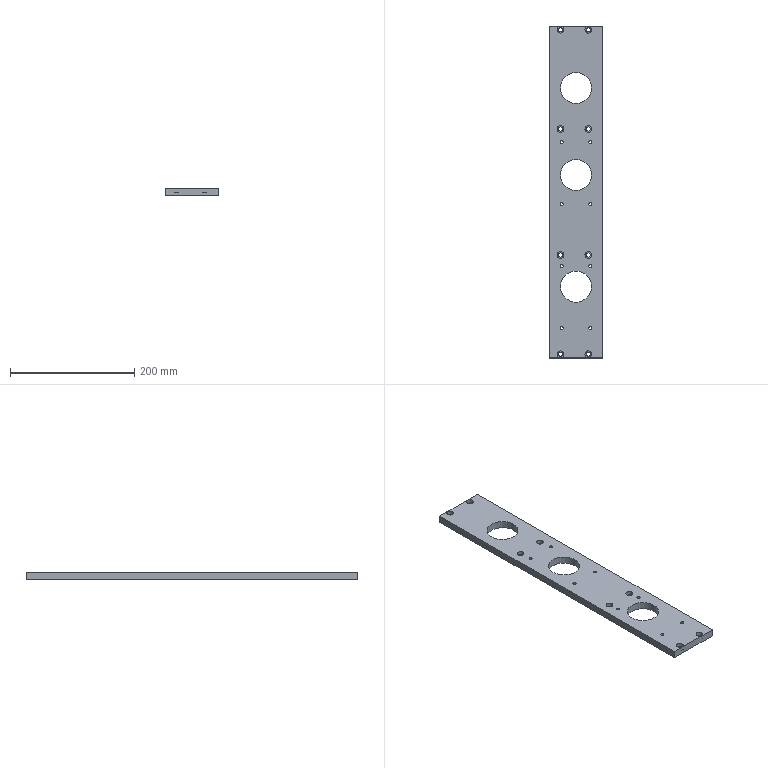Part | NX | 1 solid | 51 faces | box 86 x 535 x 12 mm | volume 472152 mm3 | cylinder 32 | plane 14 | cone 5 | commonest cylinder face diameters 5 x8 6.6 x8 11 x8 4.2 x5 50 x3
STEP:
#1=CARTESIAN_POINT('',(43.,-257.5,-2.1));
#2=VERTEX_POINT('',#1);
#3=CARTESIAN_POINT('',(43.,-257.5,0.));
#4=DIRECTION('',(1.,0.,0.));
#5=DIRECTION('',(0.,0.,-1.));
#6=AXIS2_PLACEMENT_3D('',#3,#4,#5);
#7=CIRCLE('',#6,2.1);
#8=EDGE_CURVE('',#2,#2,#7,.T.);
#9=ORIENTED_EDGE('',*,*,#8,.F.);
#10=EDGE_LOOP('',(#9));
#11=FACE_BOUND('',#10,.T.);
#12=CARTESIAN_POINT('',(43.,-117.5,-2.1));
#13=VERTEX_POINT('',#12);
#14=CARTESIAN_POINT('',(43.,-117.5,0.));
#15=DIRECTION('',(1.,0.,0.));
#16=DIRECTION('',(0.,0.,-1.));
#17=AXIS2_PLACEMENT_3D('',#14,#15,#16);
#18=CIRCLE('',#17,2.1);
#19=EDGE_CURVE('',#13,#13,#18,.T.);
#20=ORIENTED_EDGE('',*,*,#19,.F.);
#21=EDGE_LOOP('',(#20));
#22=FACE_BOUND('',#21,.T.);
#23=CARTESIAN_POINT('',(43.,117.5,-2.1));
#24=VERTEX_POINT('',#23);
#25=CARTESIAN_POINT('',(43.,117.5,0.));
#26=DIRECTION('',(1.,0.,0.));
#27=DIRECTION('',(0.,0.,-1.));
#28=AXIS2_PLACEMENT_3D('',#25,#26,#27);
#29=CIRCLE('',#28,2.1);
#30=EDGE_CURVE('',#24,#24,#29,.T.);
#31=ORIENTED_EDGE('',*,*,#30,.F.);
#32=EDGE_LOOP('',(#31));
#33=FACE_BOUND('',#32,.T.);
#34=CARTESIAN_POINT('',(43.,257.5,-2.1));
#35=VERTEX_POINT('',#34);
#36=CARTESIAN_POINT('',(43.,257.5,0.));
#37=DIRECTION('',(1.,0.,0.));
#38=DIRECTION('',(0.,0.,-1.));
#39=AXIS2_PLACEMENT_3D('',#36,#37,#38);
#40=CIRCLE('',#39,2.1);
#41=EDGE_CURVE('',#35,#35,#40,.T.);
#42=ORIENTED_EDGE('',*,*,#41,.F.);
#43=EDGE_LOOP('',(#42));
#44=FACE_BOUND('',#43,.T.);
#45=CARTESIAN_POINT('',(43.,0.,-2.1));
#46=VERTEX_POINT('',#45);
#47=CARTESIAN_POINT('',(43.,0.,0.));
#48=DIRECTION('',(1.,0.,0.));
#49=DIRECTION('',(0.,0.,-1.));
#50=AXIS2_PLACEMENT_3D('',#47,#48,#49);
#51=CIRCLE('',#50,2.1);
#52=EDGE_CURVE('',#46,#46,#51,.T.);
#53=ORIENTED_EDGE('',*,*,#52,.F.);
#54=EDGE_LOOP('',(#53));
#55=FACE_BOUND('',#54,.T.);
#56=CARTESIAN_POINT('',(43.,-267.5,-6.));
#57=VERTEX_POINT('',#56);
#58=CARTESIAN_POINT('',(43.,267.5,-6.));
#59=VERTEX_POINT('',#58);
#60=CARTESIAN_POINT('',(43.,267.5,-6.));
#61=DIRECTION('',(0.,1.,0.));
#62=VECTOR('',#61,1000.);
#63=LINE('',#60,#62);
#64=EDGE_CURVE('',#57,#59,#63,.T.);
#65=ORIENTED_EDGE('',*,*,#64,.T.);
#66=CARTESIAN_POINT('',(43.,267.5,6.));
#67=VERTEX_POINT('',#66);
#68=CARTESIAN_POINT('',(43.,267.5,6.));
#69=DIRECTION('',(0.,0.,-1.));
#70=VECTOR('',#69,1000.);
#71=LINE('',#68,#70);
#72=EDGE_CURVE('',#67,#59,#71,.T.);
#73=ORIENTED_EDGE('',*,*,#72,.F.);
#74=CARTESIAN_POINT('',(43.,-267.5,6.));
#75=VERTEX_POINT('',#74);
#76=CARTESIAN_POINT('',(43.,267.5,6.));
#77=DIRECTION('',(0.,1.,0.));
#78=VECTOR('',#77,1000.);
#79=LINE('',#76,#78);
#80=EDGE_CURVE('',#75,#67,#79,.T.);
#81=ORIENTED_EDGE('',*,*,#80,.F.);
#82=CARTESIAN_POINT('',(43.,-267.5,6.));
#83=DIRECTION('',(0.,0.,-1.));
#84=VECTOR('',#83,1000.);
#85=LINE('',#82,#84);
#86=EDGE_CURVE('',#75,#57,#85,.T.);
#87=ORIENTED_EDGE('',*,*,#86,.T.);
#88=EDGE_LOOP('',(#65,#73,#81,#87));
#89=FACE_BOUND('',#88,.T.);
#90=CARTESIAN_POINT('',(43.,267.5,6.));
#91=DIRECTION('',(-1.,0.,0.));
#92=DIRECTION('',(0.,-1.,0.));
#93=AXIS2_PLACEMENT_3D('',#90,#91,#92);
#94=PLANE('',#93);
#95=ADVANCED_FACE('',(#11,#22,#33,#44,#55,#89),#94,.F.);
#96=CARTESIAN_POINT('',(-43.,267.5,-6.));
#97=VERTEX_POINT('',#96);
#98=CARTESIAN_POINT('',(-43.,267.5,-6.));
#99=DIRECTION('',(-1.,0.,0.));
#100=VECTOR('',#99,1000.);
#101=LINE('',#98,#100);
#102=EDGE_CURVE('',#59,#97,#101,.T.);
#103=ORIENTED_EDGE('',*,*,#102,.T.);
#104=CARTESIAN_POINT('',(-43.,267.5,6.));
#105=VERTEX_POINT('',#104);
#106=CARTESIAN_POINT('',(-43.,267.5,6.));
#107=DIRECTION('',(0.,0.,-1.));
#108=VECTOR('',#107,1000.);
#109=LINE('',#106,#108);
#110=EDGE_CURVE('',#105,#97,#109,.T.);
#111=ORIENTED_EDGE('',*,*,#110,.F.);
#112=CARTESIAN_POINT('',(-43.,267.5,6.));
#113=DIRECTION('',(-1.,0.,0.));
#114=VECTOR('',#113,1000.);
#115=LINE('',#112,#114);
#116=EDGE_CURVE('',#67,#105,#115,.T.);
#117=ORIENTED_EDGE('',*,*,#116,.F.);
#118=ORIENTED_EDGE('',*,*,#72,.T.);
#119=EDGE_LOOP('',(#103,#111,#117,#118));
#120=FACE_BOUND('',#119,.T.);
#121=CARTESIAN_POINT('',(-43.,267.5,6.));
#122=DIRECTION('',(0.,-1.,0.));
#123=DIRECTION('',(0.,0.,-1.));
#124=AXIS2_PLACEMENT_3D('',#121,#122,#123);
#125=PLANE('',#124);
#126=ADVANCED_FACE('',(#120),#125,.F.);
#127=CARTESIAN_POINT('',(-43.,-267.5,-6.));
#128=VERTEX_POINT('',#127);
#129=CARTESIAN_POINT('',(-43.,267.5,-6.));
#130=DIRECTION('',(0.,-1.,0.));
#131=VECTOR('',#130,1000.);
#132=LINE('',#129,#131);
#133=EDGE_CURVE('',#97,#128,#132,.T.);
#134=ORIENTED_EDGE('',*,*,#133,.T.);
#135=CARTESIAN_POINT('',(-43.,-267.5,6.));
#136=VERTEX_POINT('',#135);
#137=CARTESIAN_POINT('',(-43.,-267.5,6.));
#138=DIRECTION('',(0.,0.,-1.));
#139=VECTOR('',#138,1000.);
#140=LINE('',#137,#139);
#141=EDGE_CURVE('',#136,#128,#140,.T.);
#142=ORIENTED_EDGE('',*,*,#141,.F.);
#143=CARTESIAN_POINT('',(-43.,267.5,6.));
#144=DIRECTION('',(0.,-1.,0.));
#145=VECTOR('',#144,1000.);
#146=LINE('',#143,#145);
#147=EDGE_CURVE('',#105,#136,#146,.T.);
#148=ORIENTED_EDGE('',*,*,#147,.F.);
#149=ORIENTED_EDGE('',*,*,#110,.T.);
#150=EDGE_LOOP('',(#134,#142,#148,#149));
#151=FACE_BOUND('',#150,.T.);
#152=CARTESIAN_POINT('',(-43.,267.5,6.));
#153=DIRECTION('',(1.,0.,0.));
#154=DIRECTION('',(0.,1.,0.));
#155=AXIS2_PLACEMENT_3D('',#152,#153,#154);
#156=PLANE('',#155);
#157=ADVANCED_FACE('',(#151),#156,.F.);
#158=CARTESIAN_POINT('',(-43.,-267.5,-6.));
#159=DIRECTION('',(1.,0.,0.));
#160=VECTOR('',#159,1000.);
#161=LINE('',#158,#160);
#162=EDGE_CURVE('',#128,#57,#161,.T.);
#163=ORIENTED_EDGE('',*,*,#162,.T.);
#164=ORIENTED_EDGE('',*,*,#86,.F.);
#165=CARTESIAN_POINT('',(-43.,-267.5,6.));
#166=DIRECTION('',(1.,0.,0.));
#167=VECTOR('',#166,1000.);
#168=LINE('',#165,#167);
#169=EDGE_CURVE('',#136,#75,#168,.T.);
#170=ORIENTED_EDGE('',*,*,#169,.F.);
#171=ORIENTED_EDGE('',*,*,#141,.T.);
#172=EDGE_LOOP('',(#163,#164,#170,#171));
#173=FACE_BOUND('',#172,.T.);
#174=CARTESIAN_POINT('',(-43.,-267.5,6.));
#175=DIRECTION('',(0.,1.,0.));
#176=DIRECTION('',(0.,0.,1.));
#177=AXIS2_PLACEMENT_3D('',#174,#175,#176);
#178=PLANE('',#177);
#179=ADVANCED_FACE('',(#173),#178,.F.);
#180=CARTESIAN_POINT('',(-25.,-152.5,6.));
#181=VERTEX_POINT('',#180);
#182=CARTESIAN_POINT('',(0.,-152.5,6.));
#183=DIRECTION('',(0.,0.,-1.));
#184=DIRECTION('',(-1.,0.,0.));
#185=AXIS2_PLACEMENT_3D('',#182,#183,#184);
#186=CIRCLE('',#185,25.);
#187=EDGE_CURVE('',#181,#181,#186,.T.);
#188=ORIENTED_EDGE('',*,*,#187,.T.);
#189=EDGE_LOOP('',(#188));
#190=FACE_BOUND('',#189,.T.);
#191=CARTESIAN_POINT('',(-25.,27.5,6.));
#192=VERTEX_POINT('',#191);
#193=CARTESIAN_POINT('',(0.,27.5,6.));
#194=DIRECTION('',(0.,0.,-1.));
#195=DIRECTION('',(-1.,0.,0.));
#196=AXIS2_PLACEMENT_3D('',#193,#194,#195);
#197=CIRCLE('',#196,25.);
#198=EDGE_CURVE('',#192,#192,#197,.T.);
#199=ORIENTED_EDGE('',*,*,#198,.T.);
#200=EDGE_LOOP('',(#199));
#201=FACE_BOUND('',#200,.T.);
#202=CARTESIAN_POINT('',(-25.,167.5,6.));
#203=VERTEX_POINT('',#202);
#204=CARTESIAN_POINT('',(0.,167.5,6.));
#205=DIRECTION('',(0.,0.,-1.));
#206=DIRECTION('',(-1.,0.,0.));
#207=AXIS2_PLACEMENT_3D('',#204,#205,#206);
#208=CIRCLE('',#207,25.);
#209=EDGE_CURVE('',#203,#203,#208,.T.);
#210=ORIENTED_EDGE('',*,*,#209,.T.);
#211=EDGE_LOOP('',(#210));
#212=FACE_BOUND('',#211,.T.);
#213=CARTESIAN_POINT('',(-19.5,101.5,6.));
#214=VERTEX_POINT('',#213);
#215=CARTESIAN_POINT('',(-25.,101.5,6.));
#216=DIRECTION('',(0.,0.,1.));
#217=DIRECTION('',(1.,0.,0.));
#218=AXIS2_PLACEMENT_3D('',#215,#216,#217);
#219=CIRCLE('',#218,5.5);
#220=EDGE_CURVE('',#214,#214,#219,.T.);
#221=ORIENTED_EDGE('',*,*,#220,.F.);
#222=EDGE_LOOP('',(#221));
#223=FACE_BOUND('',#222,.T.);
#224=CARTESIAN_POINT('',(25.5,101.5,6.));
#225=VERTEX_POINT('',#224);
#226=CARTESIAN_POINT('',(20.,101.5,6.));
#227=DIRECTION('',(0.,0.,1.));
#228=DIRECTION('',(1.,0.,0.));
#229=AXIS2_PLACEMENT_3D('',#226,#227,#228);
#230=CIRCLE('',#229,5.5);
#231=EDGE_CURVE('',#225,#225,#230,.T.);
#232=ORIENTED_EDGE('',*,*,#231,.F.);
#233=EDGE_LOOP('',(#232));
#234=FACE_BOUND('',#233,.T.);
#235=CARTESIAN_POINT('',(-19.5,-101.5,6.));
#236=VERTEX_POINT('',#235);
#237=CARTESIAN_POINT('',(-25.,-101.5,6.));
#238=DIRECTION('',(0.,0.,1.));
#239=DIRECTION('',(1.,0.,0.));
#240=AXIS2_PLACEMENT_3D('',#237,#238,#239);
#241=CIRCLE('',#240,5.5);
#242=EDGE_CURVE('',#236,#236,#241,.T.);
#243=ORIENTED_EDGE('',*,*,#242,.F.);
#244=EDGE_LOOP('',(#243));
#245=FACE_BOUND('',#244,.T.);
#246=CARTESIAN_POINT('',(25.5,-101.5,6.));
#247=VERTEX_POINT('',#246);
#248=CARTESIAN_POINT('',(20.,-101.5,6.));
#249=DIRECTION('',(0.,0.,1.));
#250=DIRECTION('',(1.,0.,0.));
#251=AXIS2_PLACEMENT_3D('',#248,#249,#250);
#252=CIRCLE('',#251,5.5);
#253=EDGE_CURVE('',#247,#247,#252,.T.);
#254=ORIENTED_EDGE('',*,*,#253,.F.);
#255=EDGE_LOOP('',(#254));
#256=FACE_BOUND('',#255,.T.);
#257=CARTESIAN_POINT('',(-19.5,-261.5,6.));
#258=VERTEX_POINT('',#257);
#259=CARTESIAN_POINT('',(-25.,-261.5,6.));
#260=DIRECTION('',(0.,0.,1.));
#261=DIRECTION('',(1.,0.,0.));
#262=AXIS2_PLACEMENT_3D('',#259,#260,#261);
#263=CIRCLE('',#262,5.5);
#264=EDGE_CURVE('',#258,#258,#263,.T.);
#265=ORIENTED_EDGE('',*,*,#264,.F.);
#266=EDGE_LOOP('',(#265));
#267=FACE_BOUND('',#266,.T.);
#268=CARTESIAN_POINT('',(25.5,-261.5,6.));
#269=VERTEX_POINT('',#268);
#270=CARTESIAN_POINT('',(20.,-261.5,6.));
#271=DIRECTION('',(0.,0.,1.));
#272=DIRECTION('',(1.,0.,0.));
#273=AXIS2_PLACEMENT_3D('',#270,#271,#272);
#274=CIRCLE('',#273,5.5);
#275=EDGE_CURVE('',#269,#269,#274,.T.);
#276=ORIENTED_EDGE('',*,*,#275,.F.);
#277=EDGE_LOOP('',(#276));
#278=FACE_BOUND('',#277,.T.);
#279=CARTESIAN_POINT('',(25.5,261.5,6.));
#280=VERTEX_POINT('',#279);
#281=CARTESIAN_POINT('',(20.,261.5,6.));
#282=DIRECTION('',(0.,0.,1.));
#283=DIRECTION('',(1.,0.,0.));
#284=AXIS2_PLACEMENT_3D('',#281,#282,#283);
#285=CIRCLE('',#284,5.5);
#286=EDGE_CURVE('',#280,#280,#285,.T.);
#287=ORIENTED_EDGE('',*,*,#286,.F.);
#288=EDGE_LOOP('',(#287));
#289=FACE_BOUND('',#288,.T.);
#290=CARTESIAN_POINT('',(-19.5,261.5,6.));
#291=VERTEX_POINT('',#290);
#292=CARTESIAN_POINT('',(-25.,261.5,6.));
#293=DIRECTION('',(0.,0.,1.));
#294=DIRECTION('',(1.,0.,0.));
#295=AXIS2_PLACEMENT_3D('',#292,#293,#294);
#296=CIRCLE('',#295,5.5);
#297=EDGE_CURVE('',#291,#291,#296,.T.);
#298=ORIENTED_EDGE('',*,*,#297,.F.);
#299=EDGE_LOOP('',(#298));
#300=FACE_BOUND('',#299,.T.);
#301=CARTESIAN_POINT('',(25.5,-19.5,6.));
#302=VERTEX_POINT('',#301);
#303=CARTESIAN_POINT('',(23.,-19.5,6.));
#304=DIRECTION('',(0.,0.,1.));
#305=DIRECTION('',(1.,0.,0.));
#306=AXIS2_PLACEMENT_3D('',#303,#304,#305);
#307=CIRCLE('',#306,2.5);
#308=EDGE_CURVE('',#302,#302,#307,.T.);
#309=ORIENTED_EDGE('',*,*,#308,.F.);
#310=EDGE_LOOP('',(#309));
#311=FACE_BOUND('',#310,.T.);
#312=CARTESIAN_POINT('',(-20.5,-19.5,6.));
#313=VERTEX_POINT('',#312);
#314=CARTESIAN_POINT('',(-23.,-19.5,6.));
#315=DIRECTION('',(0.,0.,1.));
#316=DIRECTION('',(1.,0.,0.));
#317=AXIS2_PLACEMENT_3D('',#314,#315,#316);
#318=CIRCLE('',#317,2.5);
#319=EDGE_CURVE('',#313,#313,#318,.T.);
#320=ORIENTED_EDGE('',*,*,#319,.F.);
#321=EDGE_LOOP('',(#320));
#322=FACE_BOUND('',#321,.T.);
#323=CARTESIAN_POINT('',(-20.5,80.5,6.));
#324=VERTEX_POINT('',#323);
#325=CARTESIAN_POINT('',(-23.,80.5,6.));
#326=DIRECTION('',(0.,0.,1.));
#327=DIRECTION('',(1.,0.,0.));
#328=AXIS2_PLACEMENT_3D('',#325,#326,#327);
#329=CIRCLE('',#328,2.5);
#330=EDGE_CURVE('',#324,#324,#329,.T.);
#331=ORIENTED_EDGE('',*,*,#330,.F.);
#332=EDGE_LOOP('',(#331));
#333=FACE_BOUND('',#332,.T.);
#334=CARTESIAN_POINT('',(25.5,80.5,6.));
#335=VERTEX_POINT('',#334);
#336=CARTESIAN_POINT('',(23.,80.5,6.));
#337=DIRECTION('',(0.,0.,1.));
#338=DIRECTION('',(1.,0.,0.));
#339=AXIS2_PLACEMENT_3D('',#336,#337,#338);
#340=CIRCLE('',#339,2.5);
#341=EDGE_CURVE('',#335,#335,#340,.T.);
#342=ORIENTED_EDGE('',*,*,#341,.F.);
#343=EDGE_LOOP('',(#342));
#344=FACE_BOUND('',#343,.T.);
#345=ORIENTED_EDGE('',*,*,#80,.T.);
#346=ORIENTED_EDGE('',*,*,#116,.T.);
#347=ORIENTED_EDGE('',*,*,#147,.T.);
#348=ORIENTED_EDGE('',*,*,#169,.T.);
#349=EDGE_LOOP('',(#345,#346,#347,#348));
#350=FACE_BOUND('',#349,.T.);
#351=CARTESIAN_POINT('',(-20.5,-119.5,6.));
#352=VERTEX_POINT('',#351);
#353=CARTESIAN_POINT('',(-23.,-119.5,6.));
#354=DIRECTION('',(0.,0.,1.));
#355=DIRECTION('',(1.,0.,0.));
#356=AXIS2_PLACEMENT_3D('',#353,#354,#355);
#357=CIRCLE('',#356,2.5);
#358=EDGE_CURVE('',#352,#352,#357,.T.);
#359=ORIENTED_EDGE('',*,*,#358,.F.);
#360=EDGE_LOOP('',(#359));
#361=FACE_BOUND('',#360,.T.);
#362=CARTESIAN_POINT('',(-20.5,-219.5,6.));
#363=VERTEX_POINT('',#362);
#364=CARTESIAN_POINT('',(-23.,-219.5,6.));
#365=DIRECTION('',(0.,0.,1.));
#366=DIRECTION('',(1.,0.,0.));
#367=AXIS2_PLACEMENT_3D('',#364,#365,#366);
#368=CIRCLE('',#367,2.5);
#369=EDGE_CURVE('',#363,#363,#368,.T.);
#370=ORIENTED_EDGE('',*,*,#369,.F.);
#371=EDGE_LOOP('',(#370));
#372=FACE_BOUND('',#371,.T.);
#373=CARTESIAN_POINT('',(25.5,-119.5,6.));
#374=VERTEX_POINT('',#373);
#375=CARTESIAN_POINT('',(23.,-119.5,6.));
#376=DIRECTION('',(0.,0.,1.));
#377=DIRECTION('',(1.,0.,0.));
#378=AXIS2_PLACEMENT_3D('',#375,#376,#377);
#379=CIRCLE('',#378,2.5);
#380=EDGE_CURVE('',#374,#374,#379,.T.);
#381=ORIENTED_EDGE('',*,*,#380,.F.);
#382=EDGE_LOOP('',(#381));
#383=FACE_BOUND('',#382,.T.);
#384=CARTESIAN_POINT('',(25.5,-219.5,6.));
#385=VERTEX_POINT('',#384);
#386=CARTESIAN_POINT('',(23.,-219.5,6.));
#387=DIRECTION('',(0.,0.,1.));
#388=DIRECTION('',(1.,0.,0.));
#389=AXIS2_PLACEMENT_3D('',#386,#387,#388);
#390=CIRCLE('',#389,2.5);
#391=EDGE_CURVE('',#385,#385,#390,.T.);
#392=ORIENTED_EDGE('',*,*,#391,.F.);
#393=EDGE_LOOP('',(#392));
#394=FACE_BOUND('',#393,.T.);
#395=CARTESIAN_POINT('',(0.,0.,6.));
#396=DIRECTION('',(0.,0.,1.));
#397=DIRECTION('',(1.,0.,0.));
#398=AXIS2_PLACEMENT_3D('',#395,#396,#397);
#399=PLANE('',#398);
#400=ADVANCED_FACE('',(#190,#201,#212,#223,#234,#245,#256,#267,#278,#289,#300,#311,#322,#333,#344,#350,#361,#372,#383,#394),#399,.T.);
#401=CARTESIAN_POINT('',(-25.,-152.5,-6.));
#402=VERTEX_POINT('',#401);
#403=CARTESIAN_POINT('',(0.,-152.5,-6.));
#404=DIRECTION('',(0.,0.,-1.));
#405=DIRECTION('',(-1.,0.,0.));
#406=AXIS2_PLACEMENT_3D('',#403,#404,#405);
#407=CIRCLE('',#406,25.);
#408=EDGE_CURVE('',#402,#402,#407,.T.);
#409=ORIENTED_EDGE('',*,*,#408,.F.);
#410=EDGE_LOOP('',(#409));
#411=FACE_BOUND('',#410,.T.);
#412=CARTESIAN_POINT('',(-25.,27.5,-6.));
#413=VERTEX_POINT('',#412);
#414=CARTESIAN_POINT('',(0.,27.5,-6.));
#415=DIRECTION('',(0.,0.,-1.));
#416=DIRECTION('',(-1.,0.,0.));
#417=AXIS2_PLACEMENT_3D('',#414,#415,#416);
#418=CIRCLE('',#417,25.);
#419=EDGE_CURVE('',#413,#413,#418,.T.);
#420=ORIENTED_EDGE('',*,*,#419,.F.);
#421=EDGE_LOOP('',(#420));
#422=FACE_BOUND('',#421,.T.);
#423=CARTESIAN_POINT('',(-25.,167.5,-6.));
#424=VERTEX_POINT('',#423);
#425=CARTESIAN_POINT('',(0.,167.5,-6.));
#426=DIRECTION('',(0.,0.,-1.));
#427=DIRECTION('',(-1.,0.,0.));
#428=AXIS2_PLACEMENT_3D('',#425,#426,#427);
#429=CIRCLE('',#428,25.);
#430=EDGE_CURVE('',#424,#424,#429,.T.);
#431=ORIENTED_EDGE('',*,*,#430,.F.);
#432=EDGE_LOOP('',(#431));
#433=FACE_BOUND('',#432,.T.);
#434=CARTESIAN_POINT('',(-21.7,101.5,-6.));
#435=VERTEX_POINT('',#434);
#436=CARTESIAN_POINT('',(-25.,101.5,-6.));
#437=DIRECTION('',(0.,0.,1.));
#438=DIRECTION('',(1.,0.,0.));
#439=AXIS2_PLACEMENT_3D('',#436,#437,#438);
#440=CIRCLE('',#439,3.3);
#441=EDGE_CURVE('',#435,#435,#440,.T.);
#442=ORIENTED_EDGE('',*,*,#441,.T.);
#443=EDGE_LOOP('',(#442));
#444=FACE_BOUND('',#443,.T.);
#445=CARTESIAN_POINT('',(23.3,101.5,-6.));
#446=VERTEX_POINT('',#445);
#447=CARTESIAN_POINT('',(20.,101.5,-6.));
#448=DIRECTION('',(0.,0.,1.));
#449=DIRECTION('',(1.,0.,0.));
#450=AXIS2_PLACEMENT_3D('',#447,#448,#449);
#451=CIRCLE('',#450,3.3);
#452=EDGE_CURVE('',#446,#446,#451,.T.);
#453=ORIENTED_EDGE('',*,*,#452,.T.);
#454=EDGE_LOOP('',(#453));
#455=FACE_BOUND('',#454,.T.);
#456=CARTESIAN_POINT('',(-21.7,-101.5,-6.));
#457=VERTEX_POINT('',#456);
#458=CARTESIAN_POINT('',(-25.,-101.5,-6.));
#459=DIRECTION('',(0.,0.,1.));
#460=DIRECTION('',(1.,0.,0.));
#461=AXIS2_PLACEMENT_3D('',#458,#459,#460);
#462=CIRCLE('',#461,3.3);
#463=EDGE_CURVE('',#457,#457,#462,.T.);
#464=ORIENTED_EDGE('',*,*,#463,.T.);
#465=EDGE_LOOP('',(#464));
#466=FACE_BOUND('',#465,.T.);
#467=CARTESIAN_POINT('',(23.3,-101.5,-6.));
#468=VERTEX_POINT('',#467);
#469=CARTESIAN_POINT('',(20.,-101.5,-6.));
#470=DIRECTION('',(0.,0.,1.));
#471=DIRECTION('',(1.,0.,0.));
#472=AXIS2_PLACEMENT_3D('',#469,#470,#471);
#473=CIRCLE('',#472,3.3);
#474=EDGE_CURVE('',#468,#468,#473,.T.);
#475=ORIENTED_EDGE('',*,*,#474,.T.);
#476=EDGE_LOOP('',(#475));
#477=FACE_BOUND('',#476,.T.);
#478=CARTESIAN_POINT('',(-21.7,-261.5,-6.));
#479=VERTEX_POINT('',#478);
#480=CARTESIAN_POINT('',(-25.,-261.5,-6.));
#481=DIRECTION('',(0.,0.,1.));
#482=DIRECTION('',(1.,0.,0.));
#483=AXIS2_PLACEMENT_3D('',#480,#481,#482);
#484=CIRCLE('',#483,3.3);
#485=EDGE_CURVE('',#479,#479,#484,.T.);
#486=ORIENTED_EDGE('',*,*,#485,.T.);
#487=EDGE_LOOP('',(#486));
#488=FACE_BOUND('',#487,.T.);
#489=CARTESIAN_POINT('',(23.3,-261.5,-6.));
#490=VERTEX_POINT('',#489);
#491=CARTESIAN_POINT('',(20.,-261.5,-6.));
#492=DIRECTION('',(0.,0.,1.));
#493=DIRECTION('',(1.,0.,0.));
#494=AXIS2_PLACEMENT_3D('',#491,#492,#493);
#495=CIRCLE('',#494,3.3);
#496=EDGE_CURVE('',#490,#490,#495,.T.);
#497=ORIENTED_EDGE('',*,*,#496,.T.);
#498=EDGE_LOOP('',(#497));
#499=FACE_BOUND('',#498,.T.);
#500=CARTESIAN_POINT('',(23.3,261.5,-6.));
#501=VERTEX_POINT('',#500);
#502=CARTESIAN_POINT('',(20.,261.5,-6.));
#503=DIRECTION('',(0.,0.,1.));
#504=DIRECTION('',(1.,0.,0.));
#505=AXIS2_PLACEMENT_3D('',#502,#503,#504);
#506=CIRCLE('',#505,3.3);
#507=EDGE_CURVE('',#501,#501,#506,.T.);
#508=ORIENTED_EDGE('',*,*,#507,.T.);
#509=EDGE_LOOP('',(#508));
#510=FACE_BOUND('',#509,.T.);
#511=CARTESIAN_POINT('',(-21.7,261.5,-6.));
#512=VERTEX_POINT('',#511);
#513=CARTESIAN_POINT('',(-25.,261.5,-6.));
#514=DIRECTION('',(0.,0.,1.));
#515=DIRECTION('',(1.,0.,0.));
#516=AXIS2_PLACEMENT_3D('',#513,#514,#515);
#517=CIRCLE('',#516,3.3);
#518=EDGE_CURVE('',#512,#512,#517,.T.);
#519=ORIENTED_EDGE('',*,*,#518,.T.);
#520=EDGE_LOOP('',(#519));
#521=FACE_BOUND('',#520,.T.);
#522=CARTESIAN_POINT('',(25.5,-19.5,-6.));
#523=VERTEX_POINT('',#522);
#524=CARTESIAN_POINT('',(23.,-19.5,-6.));
#525=DIRECTION('',(0.,0.,1.));
#526=DIRECTION('',(1.,0.,0.));
#527=AXIS2_PLACEMENT_3D('',#524,#525,#526);
#528=CIRCLE('',#527,2.5);
#529=EDGE_CURVE('',#523,#523,#528,.T.);
#530=ORIENTED_EDGE('',*,*,#529,.T.);
#531=EDGE_LOOP('',(#530));
#532=FACE_BOUND('',#531,.T.);
#533=CARTESIAN_POINT('',(-20.5,-19.5,-6.));
#534=VERTEX_POINT('',#533);
#535=CARTESIAN_POINT('',(-23.,-19.5,-6.));
#536=DIRECTION('',(0.,0.,1.));
#537=DIRECTION('',(1.,0.,0.));
#538=AXIS2_PLACEMENT_3D('',#535,#536,#537);
#539=CIRCLE('',#538,2.5);
#540=EDGE_CURVE('',#534,#534,#539,.T.);
#541=ORIENTED_EDGE('',*,*,#540,.T.);
#542=EDGE_LOOP('',(#541));
#543=FACE_BOUND('',#542,.T.);
#544=CARTESIAN_POINT('',(-20.5,80.5,-6.));
#545=VERTEX_POINT('',#544);
#546=CARTESIAN_POINT('',(-23.,80.5,-6.));
#547=DIRECTION('',(0.,0.,1.));
#548=DIRECTION('',(1.,0.,0.));
#549=AXIS2_PLACEMENT_3D('',#546,#547,#548);
#550=CIRCLE('',#549,2.5);
#551=EDGE_CURVE('',#545,#545,#550,.T.);
#552=ORIENTED_EDGE('',*,*,#551,.T.);
#553=EDGE_LOOP('',(#552));
#554=FACE_BOUND('',#553,.T.);
#555=CARTESIAN_POINT('',(25.5,80.5,-6.));
#556=VERTEX_POINT('',#555);
#557=CARTESIAN_POINT('',(23.,80.5,-6.));
#558=DIRECTION('',(0.,0.,1.));
#559=DIRECTION('',(1.,0.,0.));
#560=AXIS2_PLACEMENT_3D('',#557,#558,#559);
#561=CIRCLE('',#560,2.5);
#562=EDGE_CURVE('',#556,#556,#561,.T.);
#563=ORIENTED_EDGE('',*,*,#562,.T.);
#564=EDGE_LOOP('',(#563));
#565=FACE_BOUND('',#564,.T.);
#566=ORIENTED_EDGE('',*,*,#64,.F.);
#567=ORIENTED_EDGE('',*,*,#162,.F.);
#568=ORIENTED_EDGE('',*,*,#133,.F.);
#569=ORIENTED_EDGE('',*,*,#102,.F.);
#570=EDGE_LOOP('',(#566,#567,#568,#569));
#571=FACE_BOUND('',#570,.T.);
#572=CARTESIAN_POINT('',(-20.5,-119.5,-6.));
#573=VERTEX_POINT('',#572);
#574=CARTESIAN_POINT('',(-23.,-119.5,-6.));
#575=DIRECTION('',(0.,0.,1.));
#576=DIRECTION('',(1.,0.,0.));
#577=AXIS2_PLACEMENT_3D('',#574,#575,#576);
#578=CIRCLE('',#577,2.5);
#579=EDGE_CURVE('',#573,#573,#578,.T.);
#580=ORIENTED_EDGE('',*,*,#579,.T.);
#581=EDGE_LOOP('',(#580));
#582=FACE_BOUND('',#581,.T.);
#583=CARTESIAN_POINT('',(-20.5,-219.5,-6.));
#584=VERTEX_POINT('',#583);
#585=CARTESIAN_POINT('',(-23.,-219.5,-6.));
#586=DIRECTION('',(0.,0.,1.));
#587=DIRECTION('',(1.,0.,0.));
#588=AXIS2_PLACEMENT_3D('',#585,#586,#587);
#589=CIRCLE('',#588,2.5);
#590=EDGE_CURVE('',#584,#584,#589,.T.);
#591=ORIENTED_EDGE('',*,*,#590,.T.);
#592=EDGE_LOOP('',(#591));
#593=FACE_BOUND('',#592,.T.);
#594=CARTESIAN_POINT('',(25.5,-119.5,-6.));
#595=VERTEX_POINT('',#594);
#596=CARTESIAN_POINT('',(23.,-119.5,-6.));
#597=DIRECTION('',(0.,0.,1.));
#598=DIRECTION('',(1.,0.,0.));
#599=AXIS2_PLACEMENT_3D('',#596,#597,#598);
#600=CIRCLE('',#599,2.5);
#601=EDGE_CURVE('',#595,#595,#600,.T.);
#602=ORIENTED_EDGE('',*,*,#601,.T.);
#603=EDGE_LOOP('',(#602));
#604=FACE_BOUND('',#603,.T.);
#605=CARTESIAN_POINT('',(25.5,-219.5,-6.));
#606=VERTEX_POINT('',#605);
#607=CARTESIAN_POINT('',(23.,-219.5,-6.));
#608=DIRECTION('',(0.,0.,1.));
#609=DIRECTION('',(1.,0.,0.));
#610=AXIS2_PLACEMENT_3D('',#607,#608,#609);
#611=CIRCLE('',#610,2.5);
#612=EDGE_CURVE('',#606,#606,#611,.T.);
#613=ORIENTED_EDGE('',*,*,#612,.T.);
#614=EDGE_LOOP('',(#613));
#615=FACE_BOUND('',#614,.T.);
#616=CARTESIAN_POINT('',(0.,0.,-6.));
#617=DIRECTION('',(0.,0.,1.));
#618=DIRECTION('',(1.,0.,0.));
#619=AXIS2_PLACEMENT_3D('',#616,#617,#618);
#620=PLANE('',#619);
#621=ADVANCED_FACE('',(#411,#422,#433,#444,#455,#466,#477,#488,#499,#510,#521,#532,#543,#554,#565,#571,#582,#593,#604,#615),#620,.F.);
#622=ORIENTED_EDGE('',*,*,#341,.T.);
#623=EDGE_LOOP('',(#622));
#624=FACE_BOUND('',#623,.T.);
#625=ORIENTED_EDGE('',*,*,#562,.F.);
#626=EDGE_LOOP('',(#625));
#627=FACE_BOUND('',#626,.T.);
#628=CARTESIAN_POINT('',(23.,80.5,6.));
#629=DIRECTION('',(0.,0.,1.));
#630=DIRECTION('',(1.,0.,0.));
#631=AXIS2_PLACEMENT_3D('',#628,#629,#630);
#632=CYLINDRICAL_SURFACE('',#631,2.5);
#633=ADVANCED_FACE('',(#624,#627),#632,.F.);
#634=ORIENTED_EDGE('',*,*,#330,.T.);
#635=EDGE_LOOP('',(#634));
#636=FACE_BOUND('',#635,.T.);
#637=ORIENTED_EDGE('',*,*,#551,.F.);
#638=EDGE_LOOP('',(#637));
#639=FACE_BOUND('',#638,.T.);
#640=CARTESIAN_POINT('',(-23.,80.5,6.));
#641=DIRECTION('',(0.,0.,1.));
#642=DIRECTION('',(1.,0.,0.));
#643=AXIS2_PLACEMENT_3D('',#640,#641,#642);
#644=CYLINDRICAL_SURFACE('',#643,2.5);
#645=ADVANCED_FACE('',(#636,#639),#644,.F.);
#646=ORIENTED_EDGE('',*,*,#319,.T.);
#647=EDGE_LOOP('',(#646));
#648=FACE_BOUND('',#647,.T.);
#649=ORIENTED_EDGE('',*,*,#540,.F.);
#650=EDGE_LOOP('',(#649));
#651=FACE_BOUND('',#650,.T.);
#652=CARTESIAN_POINT('',(-23.,-19.5,6.));
#653=DIRECTION('',(0.,0.,1.));
#654=DIRECTION('',(1.,0.,0.));
#655=AXIS2_PLACEMENT_3D('',#652,#653,#654);
#656=CYLINDRICAL_SURFACE('',#655,2.5);
#657=ADVANCED_FACE('',(#648,#651),#656,.F.);
#658=ORIENTED_EDGE('',*,*,#358,.T.);
#659=EDGE_LOOP('',(#658));
#660=FACE_BOUND('',#659,.T.);
#661=ORIENTED_EDGE('',*,*,#579,.F.);
#662=EDGE_LOOP('',(#661));
#663=FACE_BOUND('',#662,.T.);
#664=CARTESIAN_POINT('',(-23.,-119.5,6.));
#665=DIRECTION('',(0.,0.,1.));
#666=DIRECTION('',(1.,0.,0.));
#667=AXIS2_PLACEMENT_3D('',#664,#665,#666);
#668=CYLINDRICAL_SURFACE('',#667,2.5);
#669=ADVANCED_FACE('',(#660,#663),#668,.F.);
#670=ORIENTED_EDGE('',*,*,#369,.T.);
#671=EDGE_LOOP('',(#670));
#672=FACE_BOUND('',#671,.T.);
#673=ORIENTED_EDGE('',*,*,#590,.F.);
#674=EDGE_LOOP('',(#673));
#675=FACE_BOUND('',#674,.T.);
#676=CARTESIAN_POINT('',(-23.,-219.5,6.));
#677=DIRECTION('',(0.,0.,1.));
#678=DIRECTION('',(1.,0.,0.));
#679=AXIS2_PLACEMENT_3D('',#676,#677,#678);
#680=CYLINDRICAL_SURFACE('',#679,2.5);
#681=ADVANCED_FACE('',(#672,#675),#680,.F.);
#682=ORIENTED_EDGE('',*,*,#308,.T.);
#683=EDGE_LOOP('',(#682));
#684=FACE_BOUND('',#683,.T.);
#685=ORIENTED_EDGE('',*,*,#529,.F.);
#686=EDGE_LOOP('',(#685));
#687=FACE_BOUND('',#686,.T.);
#688=CARTESIAN_POINT('',(23.,-19.5,6.));
#689=DIRECTION('',(0.,0.,1.));
#690=DIRECTION('',(1.,0.,0.));
#691=AXIS2_PLACEMENT_3D('',#688,#689,#690);
#692=CYLINDRICAL_SURFACE('',#691,2.5);
#693=ADVANCED_FACE('',(#684,#687),#692,.F.);
#694=ORIENTED_EDGE('',*,*,#380,.T.);
#695=EDGE_LOOP('',(#694));
#696=FACE_BOUND('',#695,.T.);
#697=ORIENTED_EDGE('',*,*,#601,.F.);
#698=EDGE_LOOP('',(#697));
#699=FACE_BOUND('',#698,.T.);
#700=CARTESIAN_POINT('',(23.,-119.5,6.));
#701=DIRECTION('',(0.,0.,1.));
#702=DIRECTION('',(1.,0.,0.));
#703=AXIS2_PLACEMENT_3D('',#700,#701,#702);
#704=CYLINDRICAL_SURFACE('',#703,2.5);
#705=ADVANCED_FACE('',(#696,#699),#704,.F.);
#706=ORIENTED_EDGE('',*,*,#391,.T.);
#707=EDGE_LOOP('',(#706));
#708=FACE_BOUND('',#707,.T.);
#709=ORIENTED_EDGE('',*,*,#612,.F.);
#710=EDGE_LOOP('',(#709));
#711=FACE_BOUND('',#710,.T.);
#712=CARTESIAN_POINT('',(23.,-219.5,6.));
#713=DIRECTION('',(0.,0.,1.));
#714=DIRECTION('',(1.,0.,0.));
#715=AXIS2_PLACEMENT_3D('',#712,#713,#714);
#716=CYLINDRICAL_SURFACE('',#715,2.5);
#717=ADVANCED_FACE('',(#708,#711),#716,.F.);
#718=ORIENTED_EDGE('',*,*,#518,.F.);
#719=EDGE_LOOP('',(#718));
#720=FACE_BOUND('',#719,.T.);
#721=CARTESIAN_POINT('',(-21.7,261.5,-0.4));
#722=VERTEX_POINT('',#721);
#723=CARTESIAN_POINT('',(-25.,261.5,-0.4));
#724=DIRECTION('',(0.,0.,1.));
#725=DIRECTION('',(1.,0.,0.));
#726=AXIS2_PLACEMENT_3D('',#723,#724,#725);
#727=CIRCLE('',#726,3.3);
#728=EDGE_CURVE('',#722,#722,#727,.T.);
#729=ORIENTED_EDGE('',*,*,#728,.T.);
#730=EDGE_LOOP('',(#729));
#731=FACE_BOUND('',#730,.T.);
#732=CARTESIAN_POINT('',(-25.,261.5,6.));
#733=DIRECTION('',(0.,0.,1.));
#734=DIRECTION('',(1.,0.,0.));
#735=AXIS2_PLACEMENT_3D('',#732,#733,#734);
#736=CYLINDRICAL_SURFACE('',#735,3.3);
#737=ADVANCED_FACE('',(#720,#731),#736,.F.);
#738=ORIENTED_EDGE('',*,*,#728,.F.);
#739=EDGE_LOOP('',(#738));
#740=FACE_BOUND('',#739,.T.);
#741=CARTESIAN_POINT('',(-19.5,261.5,-0.4));
#742=VERTEX_POINT('',#741);
#743=CARTESIAN_POINT('',(-25.,261.5,-0.4));
#744=DIRECTION('',(0.,0.,1.));
#745=DIRECTION('',(1.,0.,0.));
#746=AXIS2_PLACEMENT_3D('',#743,#744,#745);
#747=CIRCLE('',#746,5.5);
#748=EDGE_CURVE('',#742,#742,#747,.T.);
#749=ORIENTED_EDGE('',*,*,#748,.T.);
#750=EDGE_LOOP('',(#749));
#751=FACE_BOUND('',#750,.T.);
#752=CARTESIAN_POINT('',(-21.7,261.5,-0.4));
#753=DIRECTION('',(0.,0.,-1.));
#754=DIRECTION('',(-1.,0.,0.));
#755=AXIS2_PLACEMENT_3D('',#752,#753,#754);
#756=PLANE('',#755);
#757=ADVANCED_FACE('',(#740,#751),#756,.F.);
#758=ORIENTED_EDGE('',*,*,#748,.F.);
#759=EDGE_LOOP('',(#758));
#760=FACE_BOUND('',#759,.T.);
#761=ORIENTED_EDGE('',*,*,#297,.T.);
#762=EDGE_LOOP('',(#761));
#763=FACE_BOUND('',#762,.T.);
#764=CARTESIAN_POINT('',(-25.,261.5,6.));
#765=DIRECTION('',(0.,0.,1.));
#766=DIRECTION('',(1.,0.,0.));
#767=AXIS2_PLACEMENT_3D('',#764,#765,#766);
#768=CYLINDRICAL_SURFACE('',#767,5.5);
#769=ADVANCED_FACE('',(#760,#763),#768,.F.);
#770=ORIENTED_EDGE('',*,*,#507,.F.);
#771=EDGE_LOOP('',(#770));
#772=FACE_BOUND('',#771,.T.);
#773=CARTESIAN_POINT('',(23.3,261.5,-0.4));
#774=VERTEX_POINT('',#773);
#775=CARTESIAN_POINT('',(20.,261.5,-0.4));
#776=DIRECTION('',(0.,0.,1.));
#777=DIRECTION('',(1.,0.,0.));
#778=AXIS2_PLACEMENT_3D('',#775,#776,#777);
#779=CIRCLE('',#778,3.3);
#780=EDGE_CURVE('',#774,#774,#779,.T.);
#781=ORIENTED_EDGE('',*,*,#780,.T.);
#782=EDGE_LOOP('',(#781));
#783=FACE_BOUND('',#782,.T.);
#784=CARTESIAN_POINT('',(20.,261.5,6.));
#785=DIRECTION('',(0.,0.,1.));
#786=DIRECTION('',(1.,0.,0.));
#787=AXIS2_PLACEMENT_3D('',#784,#785,#786);
#788=CYLINDRICAL_SURFACE('',#787,3.3);
#789=ADVANCED_FACE('',(#772,#783),#788,.F.);
#790=ORIENTED_EDGE('',*,*,#780,.F.);
#791=EDGE_LOOP('',(#790));
#792=FACE_BOUND('',#791,.T.);
#793=CARTESIAN_POINT('',(25.5,261.5,-0.4));
#794=VERTEX_POINT('',#793);
#795=CARTESIAN_POINT('',(20.,261.5,-0.4));
#796=DIRECTION('',(0.,0.,1.));
#797=DIRECTION('',(1.,0.,0.));
#798=AXIS2_PLACEMENT_3D('',#795,#796,#797);
#799=CIRCLE('',#798,5.5);
#800=EDGE_CURVE('',#794,#794,#799,.T.);
#801=ORIENTED_EDGE('',*,*,#800,.T.);
#802=EDGE_LOOP('',(#801));
#803=FACE_BOUND('',#802,.T.);
#804=CARTESIAN_POINT('',(23.3,261.5,-0.4));
#805=DIRECTION('',(0.,0.,-1.));
#806=DIRECTION('',(-1.,0.,0.));
#807=AXIS2_PLACEMENT_3D('',#804,#805,#806);
#808=PLANE('',#807);
#809=ADVANCED_FACE('',(#792,#803),#808,.F.);
#810=ORIENTED_EDGE('',*,*,#800,.F.);
#811=EDGE_LOOP('',(#810));
#812=FACE_BOUND('',#811,.T.);
#813=ORIENTED_EDGE('',*,*,#286,.T.);
#814=EDGE_LOOP('',(#813));
#815=FACE_BOUND('',#814,.T.);
#816=CARTESIAN_POINT('',(20.,261.5,6.));
#817=DIRECTION('',(0.,0.,1.));
#818=DIRECTION('',(1.,0.,0.));
#819=AXIS2_PLACEMENT_3D('',#816,#817,#818);
#820=CYLINDRICAL_SURFACE('',#819,5.5);
#821=ADVANCED_FACE('',(#812,#815),#820,.F.);
#822=ORIENTED_EDGE('',*,*,#496,.F.);
#823=EDGE_LOOP('',(#822));
#824=FACE_BOUND('',#823,.T.);
#825=CARTESIAN_POINT('',(23.3,-261.5,-0.4));
#826=VERTEX_POINT('',#825);
#827=CARTESIAN_POINT('',(20.,-261.5,-0.4));
#828=DIRECTION('',(0.,0.,1.));
#829=DIRECTION('',(1.,0.,0.));
#830=AXIS2_PLACEMENT_3D('',#827,#828,#829);
#831=CIRCLE('',#830,3.3);
#832=EDGE_CURVE('',#826,#826,#831,.T.);
#833=ORIENTED_EDGE('',*,*,#832,.T.);
#834=EDGE_LOOP('',(#833));
#835=FACE_BOUND('',#834,.T.);
#836=CARTESIAN_POINT('',(20.,-261.5,6.));
#837=DIRECTION('',(0.,0.,1.));
#838=DIRECTION('',(1.,0.,0.));
#839=AXIS2_PLACEMENT_3D('',#836,#837,#838);
#840=CYLINDRICAL_SURFACE('',#839,3.3);
#841=ADVANCED_FACE('',(#824,#835),#840,.F.);
#842=ORIENTED_EDGE('',*,*,#832,.F.);
#843=EDGE_LOOP('',(#842));
#844=FACE_BOUND('',#843,.T.);
#845=CARTESIAN_POINT('',(25.5,-261.5,-0.4));
#846=VERTEX_POINT('',#845);
#847=CARTESIAN_POINT('',(20.,-261.5,-0.4));
#848=DIRECTION('',(0.,0.,1.));
#849=DIRECTION('',(1.,0.,0.));
#850=AXIS2_PLACEMENT_3D('',#847,#848,#849);
#851=CIRCLE('',#850,5.5);
#852=EDGE_CURVE('',#846,#846,#851,.T.);
#853=ORIENTED_EDGE('',*,*,#852,.T.);
#854=EDGE_LOOP('',(#853));
#855=FACE_BOUND('',#854,.T.);
#856=CARTESIAN_POINT('',(23.3,-261.5,-0.4));
#857=DIRECTION('',(0.,0.,-1.));
#858=DIRECTION('',(-1.,0.,0.));
#859=AXIS2_PLACEMENT_3D('',#856,#857,#858);
#860=PLANE('',#859);
#861=ADVANCED_FACE('',(#844,#855),#860,.F.);
#862=ORIENTED_EDGE('',*,*,#852,.F.);
#863=EDGE_LOOP('',(#862));
#864=FACE_BOUND('',#863,.T.);
#865=ORIENTED_EDGE('',*,*,#275,.T.);
#866=EDGE_LOOP('',(#865));
#867=FACE_BOUND('',#866,.T.);
#868=CARTESIAN_POINT('',(20.,-261.5,6.));
#869=DIRECTION('',(0.,0.,1.));
#870=DIRECTION('',(1.,0.,0.));
#871=AXIS2_PLACEMENT_3D('',#868,#869,#870);
#872=CYLINDRICAL_SURFACE('',#871,5.5);
#873=ADVANCED_FACE('',(#864,#867),#872,.F.);
#874=ORIENTED_EDGE('',*,*,#485,.F.);
#875=EDGE_LOOP('',(#874));
#876=FACE_BOUND('',#875,.T.);
#877=CARTESIAN_POINT('',(-21.7,-261.5,-0.4));
#878=VERTEX_POINT('',#877);
#879=CARTESIAN_POINT('',(-25.,-261.5,-0.4));
#880=DIRECTION('',(0.,0.,1.));
#881=DIRECTION('',(1.,0.,0.));
#882=AXIS2_PLACEMENT_3D('',#879,#880,#881);
#883=CIRCLE('',#882,3.3);
#884=EDGE_CURVE('',#878,#878,#883,.T.);
#885=ORIENTED_EDGE('',*,*,#884,.T.);
#886=EDGE_LOOP('',(#885));
#887=FACE_BOUND('',#886,.T.);
#888=CARTESIAN_POINT('',(-25.,-261.5,6.));
#889=DIRECTION('',(0.,0.,1.));
#890=DIRECTION('',(1.,0.,0.));
#891=AXIS2_PLACEMENT_3D('',#888,#889,#890);
#892=CYLINDRICAL_SURFACE('',#891,3.3);
#893=ADVANCED_FACE('',(#876,#887),#892,.F.);
#894=ORIENTED_EDGE('',*,*,#884,.F.);
#895=EDGE_LOOP('',(#894));
#896=FACE_BOUND('',#895,.T.);
#897=CARTESIAN_POINT('',(-19.5,-261.5,-0.4));
#898=VERTEX_POINT('',#897);
#899=CARTESIAN_POINT('',(-25.,-261.5,-0.4));
#900=DIRECTION('',(0.,0.,1.));
#901=DIRECTION('',(1.,0.,0.));
#902=AXIS2_PLACEMENT_3D('',#899,#900,#901);
#903=CIRCLE('',#902,5.5);
#904=EDGE_CURVE('',#898,#898,#903,.T.);
#905=ORIENTED_EDGE('',*,*,#904,.T.);
#906=EDGE_LOOP('',(#905));
#907=FACE_BOUND('',#906,.T.);
#908=CARTESIAN_POINT('',(-21.7,-261.5,-0.4));
#909=DIRECTION('',(0.,0.,-1.));
#910=DIRECTION('',(-1.,0.,0.));
#911=AXIS2_PLACEMENT_3D('',#908,#909,#910);
#912=PLANE('',#911);
#913=ADVANCED_FACE('',(#896,#907),#912,.F.);
#914=ORIENTED_EDGE('',*,*,#904,.F.);
#915=EDGE_LOOP('',(#914));
#916=FACE_BOUND('',#915,.T.);
#917=ORIENTED_EDGE('',*,*,#264,.T.);
#918=EDGE_LOOP('',(#917));
#919=FACE_BOUND('',#918,.T.);
#920=CARTESIAN_POINT('',(-25.,-261.5,6.));
#921=DIRECTION('',(0.,0.,1.));
#922=DIRECTION('',(1.,0.,0.));
#923=AXIS2_PLACEMENT_3D('',#920,#921,#922);
#924=CYLINDRICAL_SURFACE('',#923,5.5);
#925=ADVANCED_FACE('',(#916,#919),#924,.F.);
#926=ORIENTED_EDGE('',*,*,#474,.F.);
#927=EDGE_LOOP('',(#926));
#928=FACE_BOUND('',#927,.T.);
#929=CARTESIAN_POINT('',(23.3,-101.5,-0.4));
#930=VERTEX_POINT('',#929);
#931=CARTESIAN_POINT('',(20.,-101.5,-0.4));
#932=DIRECTION('',(0.,0.,1.));
#933=DIRECTION('',(1.,0.,0.));
#934=AXIS2_PLACEMENT_3D('',#931,#932,#933);
#935=CIRCLE('',#934,3.3);
#936=EDGE_CURVE('',#930,#930,#935,.T.);
#937=ORIENTED_EDGE('',*,*,#936,.T.);
#938=EDGE_LOOP('',(#937));
#939=FACE_BOUND('',#938,.T.);
#940=CARTESIAN_POINT('',(20.,-101.5,6.));
#941=DIRECTION('',(0.,0.,1.));
#942=DIRECTION('',(1.,0.,0.));
#943=AXIS2_PLACEMENT_3D('',#940,#941,#942);
#944=CYLINDRICAL_SURFACE('',#943,3.3);
#945=ADVANCED_FACE('',(#928,#939),#944,.F.);
#946=ORIENTED_EDGE('',*,*,#936,.F.);
#947=EDGE_LOOP('',(#946));
#948=FACE_BOUND('',#947,.T.);
#949=CARTESIAN_POINT('',(25.5,-101.5,-0.4));
#950=VERTEX_POINT('',#949);
#951=CARTESIAN_POINT('',(20.,-101.5,-0.4));
#952=DIRECTION('',(0.,0.,1.));
#953=DIRECTION('',(1.,0.,0.));
#954=AXIS2_PLACEMENT_3D('',#951,#952,#953);
#955=CIRCLE('',#954,5.5);
#956=EDGE_CURVE('',#950,#950,#955,.T.);
#957=ORIENTED_EDGE('',*,*,#956,.T.);
#958=EDGE_LOOP('',(#957));
#959=FACE_BOUND('',#958,.T.);
#960=CARTESIAN_POINT('',(23.3,-101.5,-0.4));
#961=DIRECTION('',(0.,0.,-1.));
#962=DIRECTION('',(-1.,0.,0.));
#963=AXIS2_PLACEMENT_3D('',#960,#961,#962);
#964=PLANE('',#963);
#965=ADVANCED_FACE('',(#948,#959),#964,.F.);
#966=ORIENTED_EDGE('',*,*,#956,.F.);
#967=EDGE_LOOP('',(#966));
#968=FACE_BOUND('',#967,.T.);
#969=ORIENTED_EDGE('',*,*,#253,.T.);
#970=EDGE_LOOP('',(#969));
#971=FACE_BOUND('',#970,.T.);
#972=CARTESIAN_POINT('',(20.,-101.5,6.));
#973=DIRECTION('',(0.,0.,1.));
#974=DIRECTION('',(1.,0.,0.));
#975=AXIS2_PLACEMENT_3D('',#972,#973,#974);
#976=CYLINDRICAL_SURFACE('',#975,5.5);
#977=ADVANCED_FACE('',(#968,#971),#976,.F.);
#978=ORIENTED_EDGE('',*,*,#463,.F.);
#979=EDGE_LOOP('',(#978));
#980=FACE_BOUND('',#979,.T.);
#981=CARTESIAN_POINT('',(-21.7,-101.5,-0.4));
#982=VERTEX_POINT('',#981);
#983=CARTESIAN_POINT('',(-25.,-101.5,-0.4));
#984=DIRECTION('',(0.,0.,1.));
#985=DIRECTION('',(1.,0.,0.));
#986=AXIS2_PLACEMENT_3D('',#983,#984,#985);
#987=CIRCLE('',#986,3.3);
#988=EDGE_CURVE('',#982,#982,#987,.T.);
#989=ORIENTED_EDGE('',*,*,#988,.T.);
#990=EDGE_LOOP('',(#989));
#991=FACE_BOUND('',#990,.T.);
#992=CARTESIAN_POINT('',(-25.,-101.5,6.));
#993=DIRECTION('',(0.,0.,1.));
#994=DIRECTION('',(1.,0.,0.));
#995=AXIS2_PLACEMENT_3D('',#992,#993,#994);
#996=CYLINDRICAL_SURFACE('',#995,3.3);
#997=ADVANCED_FACE('',(#980,#991),#996,.F.);
#998=ORIENTED_EDGE('',*,*,#988,.F.);
#999=EDGE_LOOP('',(#998));
#1000=FACE_BOUND('',#999,.T.);
#1001=CARTESIAN_POINT('',(-19.5,-101.5,-0.4));
#1002=VERTEX_POINT('',#1001);
#1003=CARTESIAN_POINT('',(-25.,-101.5,-0.4));
#1004=DIRECTION('',(0.,0.,1.));
#1005=DIRECTION('',(1.,0.,0.));
#1006=AXIS2_PLACEMENT_3D('',#1003,#1004,#1005);
#1007=CIRCLE('',#1006,5.5);
#1008=EDGE_CURVE('',#1002,#1002,#1007,.T.);
#1009=ORIENTED_EDGE('',*,*,#1008,.T.);
#1010=EDGE_LOOP('',(#1009));
#1011=FACE_BOUND('',#1010,.T.);
#1012=CARTESIAN_POINT('',(-21.7,-101.5,-0.4));
#1013=DIRECTION('',(0.,0.,-1.));
#1014=DIRECTION('',(-1.,0.,0.));
#1015=AXIS2_PLACEMENT_3D('',#1012,#1013,#1014);
#1016=PLANE('',#1015);
#1017=ADVANCED_FACE('',(#1000,#1011),#1016,.F.);
#1018=ORIENTED_EDGE('',*,*,#1008,.F.);
#1019=EDGE_LOOP('',(#1018));
#1020=FACE_BOUND('',#1019,.T.);
#1021=ORIENTED_EDGE('',*,*,#242,.T.);
#1022=EDGE_LOOP('',(#1021));
#1023=FACE_BOUND('',#1022,.T.);
#1024=CARTESIAN_POINT('',(-25.,-101.5,6.));
#1025=DIRECTION('',(0.,0.,1.));
#1026=DIRECTION('',(1.,0.,0.));
#1027=AXIS2_PLACEMENT_3D('',#1024,#1025,#1026);
#1028=CYLINDRICAL_SURFACE('',#1027,5.5);
#1029=ADVANCED_FACE('',(#1020,#1023),#1028,.F.);
#1030=ORIENTED_EDGE('',*,*,#452,.F.);
#1031=EDGE_LOOP('',(#1030));
#1032=FACE_BOUND('',#1031,.T.);
#1033=CARTESIAN_POINT('',(23.3,101.5,-0.4));
#1034=VERTEX_POINT('',#1033);
#1035=CARTESIAN_POINT('',(20.,101.5,-0.4));
#1036=DIRECTION('',(0.,0.,1.));
#1037=DIRECTION('',(1.,0.,0.));
#1038=AXIS2_PLACEMENT_3D('',#1035,#1036,#1037);
#1039=CIRCLE('',#1038,3.3);
#1040=EDGE_CURVE('',#1034,#1034,#1039,.T.);
#1041=ORIENTED_EDGE('',*,*,#1040,.T.);
#1042=EDGE_LOOP('',(#1041));
#1043=FACE_BOUND('',#1042,.T.);
#1044=CARTESIAN_POINT('',(20.,101.5,6.));
#1045=DIRECTION('',(0.,0.,1.));
#1046=DIRECTION('',(1.,0.,0.));
#1047=AXIS2_PLACEMENT_3D('',#1044,#1045,#1046);
#1048=CYLINDRICAL_SURFACE('',#1047,3.3);
#1049=ADVANCED_FACE('',(#1032,#1043),#1048,.F.);
#1050=ORIENTED_EDGE('',*,*,#1040,.F.);
#1051=EDGE_LOOP('',(#1050));
#1052=FACE_BOUND('',#1051,.T.);
#1053=CARTESIAN_POINT('',(25.5,101.5,-0.4));
#1054=VERTEX_POINT('',#1053);
#1055=CARTESIAN_POINT('',(20.,101.5,-0.4));
#1056=DIRECTION('',(0.,0.,1.));
#1057=DIRECTION('',(1.,0.,0.));
#1058=AXIS2_PLACEMENT_3D('',#1055,#1056,#1057);
#1059=CIRCLE('',#1058,5.5);
#1060=EDGE_CURVE('',#1054,#1054,#1059,.T.);
#1061=ORIENTED_EDGE('',*,*,#1060,.T.);
#1062=EDGE_LOOP('',(#1061));
#1063=FACE_BOUND('',#1062,.T.);
#1064=CARTESIAN_POINT('',(23.3,101.5,-0.4));
#1065=DIRECTION('',(0.,0.,-1.));
#1066=DIRECTION('',(-1.,0.,0.));
#1067=AXIS2_PLACEMENT_3D('',#1064,#1065,#1066);
#1068=PLANE('',#1067);
#1069=ADVANCED_FACE('',(#1052,#1063),#1068,.F.);
#1070=ORIENTED_EDGE('',*,*,#1060,.F.);
#1071=EDGE_LOOP('',(#1070));
#1072=FACE_BOUND('',#1071,.T.);
#1073=ORIENTED_EDGE('',*,*,#231,.T.);
#1074=EDGE_LOOP('',(#1073));
#1075=FACE_BOUND('',#1074,.T.);
#1076=CARTESIAN_POINT('',(20.,101.5,6.));
#1077=DIRECTION('',(0.,0.,1.));
#1078=DIRECTION('',(1.,0.,0.));
#1079=AXIS2_PLACEMENT_3D('',#1076,#1077,#1078);
#1080=CYLINDRICAL_SURFACE('',#1079,5.5);
#1081=ADVANCED_FACE('',(#1072,#1075),#1080,.F.);
#1082=ORIENTED_EDGE('',*,*,#441,.F.);
#1083=EDGE_LOOP('',(#1082));
#1084=FACE_BOUND('',#1083,.T.);
#1085=CARTESIAN_POINT('',(-21.7,101.5,-0.4));
#1086=VERTEX_POINT('',#1085);
#1087=CARTESIAN_POINT('',(-25.,101.5,-0.4));
#1088=DIRECTION('',(0.,0.,1.));
#1089=DIRECTION('',(1.,0.,0.));
#1090=AXIS2_PLACEMENT_3D('',#1087,#1088,#1089);
#1091=CIRCLE('',#1090,3.3);
#1092=EDGE_CURVE('',#1086,#1086,#1091,.T.);
#1093=ORIENTED_EDGE('',*,*,#1092,.T.);
#1094=EDGE_LOOP('',(#1093));
#1095=FACE_BOUND('',#1094,.T.);
#1096=CARTESIAN_POINT('',(-25.,101.5,6.));
#1097=DIRECTION('',(0.,0.,1.));
#1098=DIRECTION('',(1.,0.,0.));
#1099=AXIS2_PLACEMENT_3D('',#1096,#1097,#1098);
#1100=CYLINDRICAL_SURFACE('',#1099,3.3);
#1101=ADVANCED_FACE('',(#1084,#1095),#1100,.F.);
#1102=ORIENTED_EDGE('',*,*,#1092,.F.);
#1103=EDGE_LOOP('',(#1102));
#1104=FACE_BOUND('',#1103,.T.);
#1105=CARTESIAN_POINT('',(-19.5,101.5,-0.4));
#1106=VERTEX_POINT('',#1105);
#1107=CARTESIAN_POINT('',(-25.,101.5,-0.4));
#1108=DIRECTION('',(0.,0.,1.));
#1109=DIRECTION('',(1.,0.,0.));
#1110=AXIS2_PLACEMENT_3D('',#1107,#1108,#1109);
#1111=CIRCLE('',#1110,5.5);
#1112=EDGE_CURVE('',#1106,#1106,#1111,.T.);
#1113=ORIENTED_EDGE('',*,*,#1112,.T.);
#1114=EDGE_LOOP('',(#1113));
#1115=FACE_BOUND('',#1114,.T.);
#1116=CARTESIAN_POINT('',(-21.7,101.5,-0.4));
#1117=DIRECTION('',(0.,0.,-1.));
#1118=DIRECTION('',(-1.,0.,0.));
#1119=AXIS2_PLACEMENT_3D('',#1116,#1117,#1118);
#1120=PLANE('',#1119);
#1121=ADVANCED_FACE('',(#1104,#1115),#1120,.F.);
#1122=ORIENTED_EDGE('',*,*,#1112,.F.);
#1123=EDGE_LOOP('',(#1122));
#1124=FACE_BOUND('',#1123,.T.);
#1125=ORIENTED_EDGE('',*,*,#220,.T.);
#1126=EDGE_LOOP('',(#1125));
#1127=FACE_BOUND('',#1126,.T.);
#1128=CARTESIAN_POINT('',(-25.,101.5,6.));
#1129=DIRECTION('',(0.,0.,1.));
#1130=DIRECTION('',(1.,0.,0.));
#1131=AXIS2_PLACEMENT_3D('',#1128,#1129,#1130);
#1132=CYLINDRICAL_SURFACE('',#1131,5.5);
#1133=ADVANCED_FACE('',(#1124,#1127),#1132,.F.);
#1134=ORIENTED_EDGE('',*,*,#209,.F.);
#1135=EDGE_LOOP('',(#1134));
#1136=FACE_BOUND('',#1135,.T.);
#1137=ORIENTED_EDGE('',*,*,#430,.T.);
#1138=EDGE_LOOP('',(#1137));
#1139=FACE_BOUND('',#1138,.T.);
#1140=CARTESIAN_POINT('',(0.,167.5,6.));
#1141=DIRECTION('',(0.,0.,-1.));
#1142=DIRECTION('',(-1.,0.,0.));
#1143=AXIS2_PLACEMENT_3D('',#1140,#1141,#1142);
#1144=CYLINDRICAL_SURFACE('',#1143,25.);
#1145=ADVANCED_FACE('',(#1136,#1139),#1144,.F.);
#1146=ORIENTED_EDGE('',*,*,#198,.F.);
#1147=EDGE_LOOP('',(#1146));
#1148=FACE_BOUND('',#1147,.T.);
#1149=ORIENTED_EDGE('',*,*,#419,.T.);
#1150=EDGE_LOOP('',(#1149));
#1151=FACE_BOUND('',#1150,.T.);
#1152=CARTESIAN_POINT('',(0.,27.5,6.));
#1153=DIRECTION('',(0.,0.,-1.));
#1154=DIRECTION('',(-1.,0.,0.));
#1155=AXIS2_PLACEMENT_3D('',#1152,#1153,#1154);
#1156=CYLINDRICAL_SURFACE('',#1155,25.);
#1157=ADVANCED_FACE('',(#1148,#1151),#1156,.F.);
#1158=ORIENTED_EDGE('',*,*,#187,.F.);
#1159=EDGE_LOOP('',(#1158));
#1160=FACE_BOUND('',#1159,.T.);
#1161=ORIENTED_EDGE('',*,*,#408,.T.);
#1162=EDGE_LOOP('',(#1161));
#1163=FACE_BOUND('',#1162,.T.);
#1164=CARTESIAN_POINT('',(0.,-152.5,6.));
#1165=DIRECTION('',(0.,0.,-1.));
#1166=DIRECTION('',(-1.,0.,0.));
#1167=AXIS2_PLACEMENT_3D('',#1164,#1165,#1166);
#1168=CYLINDRICAL_SURFACE('',#1167,25.);
#1169=ADVANCED_FACE('',(#1160,#1163),#1168,.F.);
#1170=CARTESIAN_POINT('',(27.738,0.,0.));
#1171=VERTEX_POINT('',#1170);
#1172=VERTEX_LOOP('',#1171);
#1173=FACE_BOUND('',#1172,.T.);
#1174=CARTESIAN_POINT('',(29.,0.,-2.1));
#1175=VERTEX_POINT('',#1174);
#1176=CARTESIAN_POINT('',(29.,0.,0.));
#1177=DIRECTION('',(1.,0.,0.));
#1178=DIRECTION('',(0.,0.,-1.));
#1179=AXIS2_PLACEMENT_3D('',#1176,#1177,#1178);
#1180=CIRCLE('',#1179,2.1);
#1181=EDGE_CURVE('',#1175,#1175,#1180,.T.);
#1182=ORIENTED_EDGE('',*,*,#1181,.T.);
#1183=EDGE_LOOP('',(#1182));
#1184=FACE_BOUND('',#1183,.T.);
#1185=CARTESIAN_POINT('',(29.,0.,0.));
#1186=DIRECTION('',(1.,0.,0.));
#1187=DIRECTION('',(0.,0.,-1.));
#1188=AXIS2_PLACEMENT_3D('',#1185,#1186,#1187);
#1189=CONICAL_SURFACE('',#1188,2.1,1.03);
#1190=ADVANCED_FACE('',(#1173,#1184),#1189,.F.);
#1191=ORIENTED_EDGE('',*,*,#1181,.F.);
#1192=EDGE_LOOP('',(#1191));
#1193=FACE_BOUND('',#1192,.T.);
#1194=ORIENTED_EDGE('',*,*,#52,.T.);
#1195=EDGE_LOOP('',(#1194));
#1196=FACE_BOUND('',#1195,.T.);
#1197=CARTESIAN_POINT('',(43.,0.,0.));
#1198=DIRECTION('',(1.,0.,0.));
#1199=DIRECTION('',(0.,0.,-1.));
#1200=AXIS2_PLACEMENT_3D('',#1197,#1198,#1199);
#1201=CYLINDRICAL_SURFACE('',#1200,2.1);
#1202=ADVANCED_FACE('',(#1193,#1196),#1201,.F.);
#1203=CARTESIAN_POINT('',(27.738,257.5,0.));
#1204=VERTEX_POINT('',#1203);
#1205=VERTEX_LOOP('',#1204);
#1206=FACE_BOUND('',#1205,.T.);
#1207=CARTESIAN_POINT('',(29.,257.5,-2.1));
#1208=VERTEX_POINT('',#1207);
#1209=CARTESIAN_POINT('',(29.,257.5,0.));
#1210=DIRECTION('',(1.,0.,0.));
#1211=DIRECTION('',(0.,0.,-1.));
#1212=AXIS2_PLACEMENT_3D('',#1209,#1210,#1211);
#1213=CIRCLE('',#1212,2.1);
#1214=EDGE_CURVE('',#1208,#1208,#1213,.T.);
#1215=ORIENTED_EDGE('',*,*,#1214,.T.);
#1216=EDGE_LOOP('',(#1215));
#1217=FACE_BOUND('',#1216,.T.);
#1218=CARTESIAN_POINT('',(29.,257.5,0.));
#1219=DIRECTION('',(1.,0.,0.));
#1220=DIRECTION('',(0.,0.,-1.));
#1221=AXIS2_PLACEMENT_3D('',#1218,#1219,#1220);
#1222=CONICAL_SURFACE('',#1221,2.1,1.03);
#1223=ADVANCED_FACE('',(#1206,#1217),#1222,.F.);
#1224=ORIENTED_EDGE('',*,*,#1214,.F.);
#1225=EDGE_LOOP('',(#1224));
#1226=FACE_BOUND('',#1225,.T.);
#1227=ORIENTED_EDGE('',*,*,#41,.T.);
#1228=EDGE_LOOP('',(#1227));
#1229=FACE_BOUND('',#1228,.T.);
#1230=CARTESIAN_POINT('',(43.,257.5,0.));
#1231=DIRECTION('',(1.,0.,0.));
#1232=DIRECTION('',(0.,0.,-1.));
#1233=AXIS2_PLACEMENT_3D('',#1230,#1231,#1232);
#1234=CYLINDRICAL_SURFACE('',#1233,2.1);
#1235=ADVANCED_FACE('',(#1226,#1229),#1234,.F.);
#1236=CARTESIAN_POINT('',(27.738,117.5,0.));
#1237=VERTEX_POINT('',#1236);
#1238=VERTEX_LOOP('',#1237);
#1239=FACE_BOUND('',#1238,.T.);
#1240=CARTESIAN_POINT('',(29.,117.5,-2.1));
#1241=VERTEX_POINT('',#1240);
#1242=CARTESIAN_POINT('',(29.,117.5,0.));
#1243=DIRECTION('',(1.,0.,0.));
#1244=DIRECTION('',(0.,0.,-1.));
#1245=AXIS2_PLACEMENT_3D('',#1242,#1243,#1244);
#1246=CIRCLE('',#1245,2.1);
#1247=EDGE_CURVE('',#1241,#1241,#1246,.T.);
#1248=ORIENTED_EDGE('',*,*,#1247,.T.);
#1249=EDGE_LOOP('',(#1248));
#1250=FACE_BOUND('',#1249,.T.);
#1251=CARTESIAN_POINT('',(29.,117.5,0.));
#1252=DIRECTION('',(1.,0.,0.));
#1253=DIRECTION('',(0.,0.,-1.));
#1254=AXIS2_PLACEMENT_3D('',#1251,#1252,#1253);
#1255=CONICAL_SURFACE('',#1254,2.1,1.03);
#1256=ADVANCED_FACE('',(#1239,#1250),#1255,.F.);
#1257=ORIENTED_EDGE('',*,*,#1247,.F.);
#1258=EDGE_LOOP('',(#1257));
#1259=FACE_BOUND('',#1258,.T.);
#1260=ORIENTED_EDGE('',*,*,#30,.T.);
#1261=EDGE_LOOP('',(#1260));
#1262=FACE_BOUND('',#1261,.T.);
#1263=CARTESIAN_POINT('',(43.,117.5,0.));
#1264=DIRECTION('',(1.,0.,0.));
#1265=DIRECTION('',(0.,0.,-1.));
#1266=AXIS2_PLACEMENT_3D('',#1263,#1264,#1265);
#1267=CYLINDRICAL_SURFACE('',#1266,2.1);
#1268=ADVANCED_FACE('',(#1259,#1262),#1267,.F.);
#1269=CARTESIAN_POINT('',(27.738,-117.5,0.));
#1270=VERTEX_POINT('',#1269);
#1271=VERTEX_LOOP('',#1270);
#1272=FACE_BOUND('',#1271,.T.);
#1273=CARTESIAN_POINT('',(29.,-117.5,-2.1));
#1274=VERTEX_POINT('',#1273);
#1275=CARTESIAN_POINT('',(29.,-117.5,0.));
#1276=DIRECTION('',(1.,0.,0.));
#1277=DIRECTION('',(0.,0.,-1.));
#1278=AXIS2_PLACEMENT_3D('',#1275,#1276,#1277);
#1279=CIRCLE('',#1278,2.1);
#1280=EDGE_CURVE('',#1274,#1274,#1279,.T.);
#1281=ORIENTED_EDGE('',*,*,#1280,.T.);
#1282=EDGE_LOOP('',(#1281));
#1283=FACE_BOUND('',#1282,.T.);
#1284=CARTESIAN_POINT('',(29.,-117.5,0.));
#1285=DIRECTION('',(1.,0.,0.));
#1286=DIRECTION('',(0.,0.,-1.));
#1287=AXIS2_PLACEMENT_3D('',#1284,#1285,#1286);
#1288=CONICAL_SURFACE('',#1287,2.1,1.03);
#1289=ADVANCED_FACE('',(#1272,#1283),#1288,.F.);
#1290=ORIENTED_EDGE('',*,*,#1280,.F.);
#1291=EDGE_LOOP('',(#1290));
#1292=FACE_BOUND('',#1291,.T.);
#1293=ORIENTED_EDGE('',*,*,#19,.T.);
#1294=EDGE_LOOP('',(#1293));
#1295=FACE_BOUND('',#1294,.T.);
#1296=CARTESIAN_POINT('',(43.,-117.5,0.));
#1297=DIRECTION('',(1.,0.,0.));
#1298=DIRECTION('',(0.,0.,-1.));
#1299=AXIS2_PLACEMENT_3D('',#1296,#1297,#1298);
#1300=CYLINDRICAL_SURFACE('',#1299,2.1);
#1301=ADVANCED_FACE('',(#1292,#1295),#1300,.F.);
#1302=CARTESIAN_POINT('',(27.738,-257.5,0.));
#1303=VERTEX_POINT('',#1302);
#1304=VERTEX_LOOP('',#1303);
#1305=FACE_BOUND('',#1304,.T.);
#1306=CARTESIAN_POINT('',(29.,-257.5,-2.1));
#1307=VERTEX_POINT('',#1306);
#1308=CARTESIAN_POINT('',(29.,-257.5,0.));
#1309=DIRECTION('',(1.,0.,0.));
#1310=DIRECTION('',(0.,0.,-1.));
#1311=AXIS2_PLACEMENT_3D('',#1308,#1309,#1310);
#1312=CIRCLE('',#1311,2.1);
#1313=EDGE_CURVE('',#1307,#1307,#1312,.T.);
#1314=ORIENTED_EDGE('',*,*,#1313,.T.);
#1315=EDGE_LOOP('',(#1314));
#1316=FACE_BOUND('',#1315,.T.);
#1317=CARTESIAN_POINT('',(29.,-257.5,0.));
#1318=DIRECTION('',(1.,0.,0.));
#1319=DIRECTION('',(0.,0.,-1.));
#1320=AXIS2_PLACEMENT_3D('',#1317,#1318,#1319);
#1321=CONICAL_SURFACE('',#1320,2.1,1.03);
#1322=ADVANCED_FACE('',(#1305,#1316),#1321,.F.);
#1323=ORIENTED_EDGE('',*,*,#1313,.F.);
#1324=EDGE_LOOP('',(#1323));
#1325=FACE_BOUND('',#1324,.T.);
#1326=ORIENTED_EDGE('',*,*,#8,.T.);
#1327=EDGE_LOOP('',(#1326));
#1328=FACE_BOUND('',#1327,.T.);
#1329=CARTESIAN_POINT('',(43.,-257.5,0.));
#1330=DIRECTION('',(1.,0.,0.));
#1331=DIRECTION('',(0.,0.,-1.));
#1332=AXIS2_PLACEMENT_3D('',#1329,#1330,#1331);
#1333=CYLINDRICAL_SURFACE('',#1332,2.1);
#1334=ADVANCED_FACE('',(#1325,#1328),#1333,.F.);
#1335=CLOSED_SHELL('',(#95,#126,#157,#179,#400,#621,#633,#645,#657,#669,#681,#693,#705,#717,#737,#757,#769,#789,#809,#821,#841,#861,#873,#893,#913,#925,#945,#965,#977,#997,#1017,#1029,#1049,#1069,#1081,#1101,#1121,#1133,#1145,#1157,#1169,#1190,#1202,#1223,#1235,#1256,#1268,#1289,#1301,#1322,#1334));
#1336=MANIFOLD_SOLID_BREP('',#1335);
#1337=(LENGTH_UNIT()NAMED_UNIT(*)SI_UNIT(.MILLI.,.METRE.));
#1338=UNCERTAINTY_MEASURE_WITH_UNIT(LENGTH_MEASURE(0.00001),#1337,'','');
#1339=(NAMED_UNIT(*)PLANE_ANGLE_UNIT()SI_UNIT($,.RADIAN.));
#1340=(NAMED_UNIT(*)SI_UNIT($,.STERADIAN.)SOLID_ANGLE_UNIT());
#1341=(GEOMETRIC_REPRESENTATION_CONTEXT(3)GLOBAL_UNCERTAINTY_ASSIGNED_CONTEXT((#1338))GLOBAL_UNIT_ASSIGNED_CONTEXT((#1337,#1339,#1340))REPRESENTATION_CONTEXT('',''));
#1342=ADVANCED_BREP_SHAPE_REPRESENTATION('',(#1336),#1341);